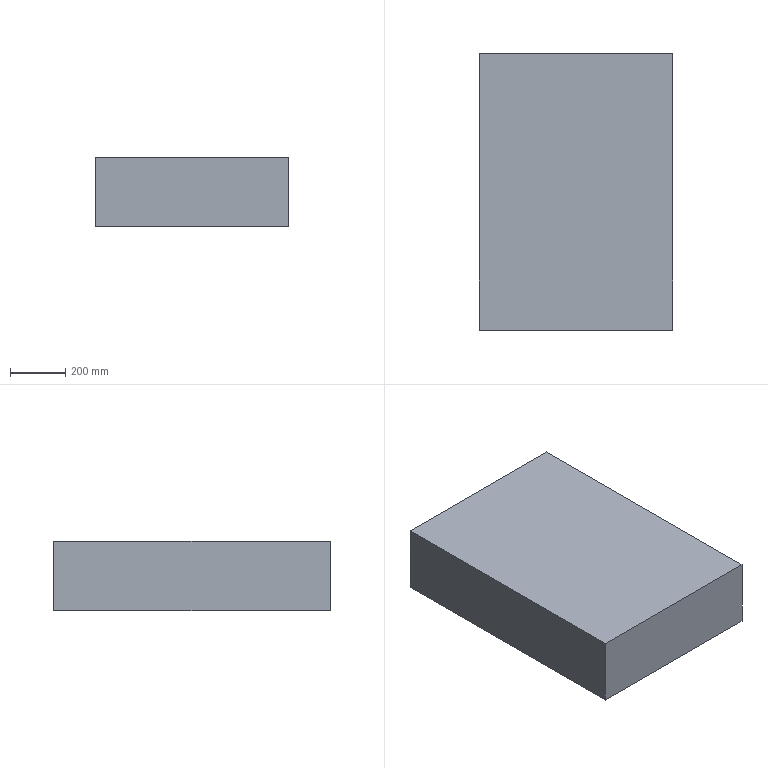Part | STEP file | BOX111 Default | 1 solid | 6 faces | box 700 x 1000 x 250 mm | volume 175000000 mm3 | plane 6
STEP:
#1=CARTESIAN_POINT('',(-350.,500.,0.));
#2=VERTEX_POINT('',#1);
#3=CARTESIAN_POINT('',(-350.,-500.,0.));
#4=VERTEX_POINT('',#3);
#5=CARTESIAN_POINT('',(-350.,-500.,0.));
#6=DIRECTION('',(0.,-1.,0.));
#7=VECTOR('',#6,1000.);
#8=LINE('',#5,#7);
#9=EDGE_CURVE('',#2,#4,#8,.T.);
#10=ORIENTED_EDGE('',*,*,#9,.T.);
#11=CARTESIAN_POINT('',(-350.,-500.,250.));
#12=VERTEX_POINT('',#11);
#13=CARTESIAN_POINT('',(-350.,-500.,250.));
#14=DIRECTION('',(0.,0.,-1.));
#15=VECTOR('',#14,1000.);
#16=LINE('',#13,#15);
#17=EDGE_CURVE('',#12,#4,#16,.T.);
#18=ORIENTED_EDGE('',*,*,#17,.F.);
#19=CARTESIAN_POINT('',(-350.,500.,250.));
#20=VERTEX_POINT('',#19);
#21=CARTESIAN_POINT('',(-350.,-500.,250.));
#22=DIRECTION('',(0.,-1.,0.));
#23=VECTOR('',#22,1000.);
#24=LINE('',#21,#23);
#25=EDGE_CURVE('',#20,#12,#24,.T.);
#26=ORIENTED_EDGE('',*,*,#25,.F.);
#27=CARTESIAN_POINT('',(-350.,500.,250.));
#28=DIRECTION('',(0.,0.,-1.));
#29=VECTOR('',#28,1000.);
#30=LINE('',#27,#29);
#31=EDGE_CURVE('',#20,#2,#30,.T.);
#32=ORIENTED_EDGE('',*,*,#31,.T.);
#33=EDGE_LOOP('',(#10,#18,#26,#32));
#34=FACE_OUTER_BOUND('',#33,.T.);
#35=CARTESIAN_POINT('',(-350.,-500.,250.));
#36=DIRECTION('',(1.,0.,0.));
#37=DIRECTION('',(0.,0.,-1.));
#38=AXIS2_PLACEMENT_3D('',#35,#36,#37);
#39=PLANE('',#38);
#40=ADVANCED_FACE('',(#34),#39,.F.);
#41=CARTESIAN_POINT('',(350.,-500.,0.));
#42=VERTEX_POINT('',#41);
#43=CARTESIAN_POINT('',(350.,-500.,0.));
#44=DIRECTION('',(1.,0.,0.));
#45=VECTOR('',#44,1000.);
#46=LINE('',#43,#45);
#47=EDGE_CURVE('',#4,#42,#46,.T.);
#48=ORIENTED_EDGE('',*,*,#47,.T.);
#49=CARTESIAN_POINT('',(350.,-500.,250.));
#50=VERTEX_POINT('',#49);
#51=CARTESIAN_POINT('',(350.,-500.,250.));
#52=DIRECTION('',(0.,0.,-1.));
#53=VECTOR('',#52,1000.);
#54=LINE('',#51,#53);
#55=EDGE_CURVE('',#50,#42,#54,.T.);
#56=ORIENTED_EDGE('',*,*,#55,.F.);
#57=CARTESIAN_POINT('',(350.,-500.,250.));
#58=DIRECTION('',(1.,0.,0.));
#59=VECTOR('',#58,1000.);
#60=LINE('',#57,#59);
#61=EDGE_CURVE('',#12,#50,#60,.T.);
#62=ORIENTED_EDGE('',*,*,#61,.F.);
#63=ORIENTED_EDGE('',*,*,#17,.T.);
#64=EDGE_LOOP('',(#48,#56,#62,#63));
#65=FACE_OUTER_BOUND('',#64,.T.);
#66=CARTESIAN_POINT('',(350.,-500.,250.));
#67=DIRECTION('',(0.,1.,0.));
#68=DIRECTION('',(-1.,0.,0.));
#69=AXIS2_PLACEMENT_3D('',#66,#67,#68);
#70=PLANE('',#69);
#71=ADVANCED_FACE('',(#65),#70,.F.);
#72=CARTESIAN_POINT('',(350.,500.,0.));
#73=VERTEX_POINT('',#72);
#74=CARTESIAN_POINT('',(350.,-500.,0.));
#75=DIRECTION('',(0.,1.,0.));
#76=VECTOR('',#75,1000.);
#77=LINE('',#74,#76);
#78=EDGE_CURVE('',#42,#73,#77,.T.);
#79=ORIENTED_EDGE('',*,*,#78,.T.);
#80=CARTESIAN_POINT('',(350.,500.,250.));
#81=VERTEX_POINT('',#80);
#82=CARTESIAN_POINT('',(350.,500.,250.));
#83=DIRECTION('',(0.,0.,-1.));
#84=VECTOR('',#83,1000.);
#85=LINE('',#82,#84);
#86=EDGE_CURVE('',#81,#73,#85,.T.);
#87=ORIENTED_EDGE('',*,*,#86,.F.);
#88=CARTESIAN_POINT('',(350.,-500.,250.));
#89=DIRECTION('',(0.,1.,0.));
#90=VECTOR('',#89,1000.);
#91=LINE('',#88,#90);
#92=EDGE_CURVE('',#50,#81,#91,.T.);
#93=ORIENTED_EDGE('',*,*,#92,.F.);
#94=ORIENTED_EDGE('',*,*,#55,.T.);
#95=EDGE_LOOP('',(#79,#87,#93,#94));
#96=FACE_OUTER_BOUND('',#95,.T.);
#97=CARTESIAN_POINT('',(350.,-500.,250.));
#98=DIRECTION('',(-1.,0.,0.));
#99=DIRECTION('',(0.,0.,1.));
#100=AXIS2_PLACEMENT_3D('',#97,#98,#99);
#101=PLANE('',#100);
#102=ADVANCED_FACE('',(#96),#101,.F.);
#103=CARTESIAN_POINT('',(350.,500.,0.));
#104=DIRECTION('',(-1.,0.,0.));
#105=VECTOR('',#104,1000.);
#106=LINE('',#103,#105);
#107=EDGE_CURVE('',#73,#2,#106,.T.);
#108=ORIENTED_EDGE('',*,*,#107,.T.);
#109=ORIENTED_EDGE('',*,*,#31,.F.);
#110=CARTESIAN_POINT('',(350.,500.,250.));
#111=DIRECTION('',(-1.,0.,0.));
#112=VECTOR('',#111,1000.);
#113=LINE('',#110,#112);
#114=EDGE_CURVE('',#81,#20,#113,.T.);
#115=ORIENTED_EDGE('',*,*,#114,.F.);
#116=ORIENTED_EDGE('',*,*,#86,.T.);
#117=EDGE_LOOP('',(#108,#109,#115,#116));
#118=FACE_OUTER_BOUND('',#117,.T.);
#119=CARTESIAN_POINT('',(350.,500.,250.));
#120=DIRECTION('',(0.,-1.,0.));
#121=DIRECTION('',(1.,0.,0.));
#122=AXIS2_PLACEMENT_3D('',#119,#120,#121);
#123=PLANE('',#122);
#124=ADVANCED_FACE('',(#118),#123,.F.);
#125=ORIENTED_EDGE('',*,*,#25,.T.);
#126=ORIENTED_EDGE('',*,*,#61,.T.);
#127=ORIENTED_EDGE('',*,*,#92,.T.);
#128=ORIENTED_EDGE('',*,*,#114,.T.);
#129=EDGE_LOOP('',(#125,#126,#127,#128));
#130=FACE_OUTER_BOUND('',#129,.T.);
#131=CARTESIAN_POINT('',(0.,0.,250.));
#132=DIRECTION('',(0.,0.,1.));
#133=DIRECTION('',(1.,0.,0.));
#134=AXIS2_PLACEMENT_3D('',#131,#132,#133);
#135=PLANE('',#134);
#136=ADVANCED_FACE('',(#130),#135,.T.);
#137=ORIENTED_EDGE('',*,*,#9,.F.);
#138=ORIENTED_EDGE('',*,*,#107,.F.);
#139=ORIENTED_EDGE('',*,*,#78,.F.);
#140=ORIENTED_EDGE('',*,*,#47,.F.);
#141=EDGE_LOOP('',(#137,#138,#139,#140));
#142=FACE_OUTER_BOUND('',#141,.T.);
#143=CARTESIAN_POINT('',(0.,0.,0.));
#144=DIRECTION('',(0.,0.,1.));
#145=DIRECTION('',(1.,0.,0.));
#146=AXIS2_PLACEMENT_3D('',#143,#144,#145);
#147=PLANE('',#146);
#148=ADVANCED_FACE('',(#142),#147,.F.);
#149=CLOSED_SHELL('',(#40,#71,#102,#124,#136,#148));
#150=MANIFOLD_SOLID_BREP('',#149);
#151=CARTESIAN_POINT('',(0.,0.,0.));
#152=DIRECTION('',(0.,0.,1.));
#153=DIRECTION('',(1.,0.,0.));
#154=AXIS2_PLACEMENT_3D('',#151,#152,#153);
#155=(LENGTH_UNIT()NAMED_UNIT(*)SI_UNIT(.MILLI.,.METRE.));
#156=UNCERTAINTY_MEASURE_WITH_UNIT(LENGTH_MEASURE(0.00001),#155,'','');
#157=(NAMED_UNIT(*)PLANE_ANGLE_UNIT()SI_UNIT($,.RADIAN.));
#158=(NAMED_UNIT(*)SI_UNIT($,.STERADIAN.)SOLID_ANGLE_UNIT());
#159=(GEOMETRIC_REPRESENTATION_CONTEXT(3)GLOBAL_UNCERTAINTY_ASSIGNED_CONTEXT((#156))GLOBAL_UNIT_ASSIGNED_CONTEXT((#155,#157,#158))REPRESENTATION_CONTEXT('',''));
#160=ADVANCED_BREP_SHAPE_REPRESENTATION('',(#150,#154),#159);